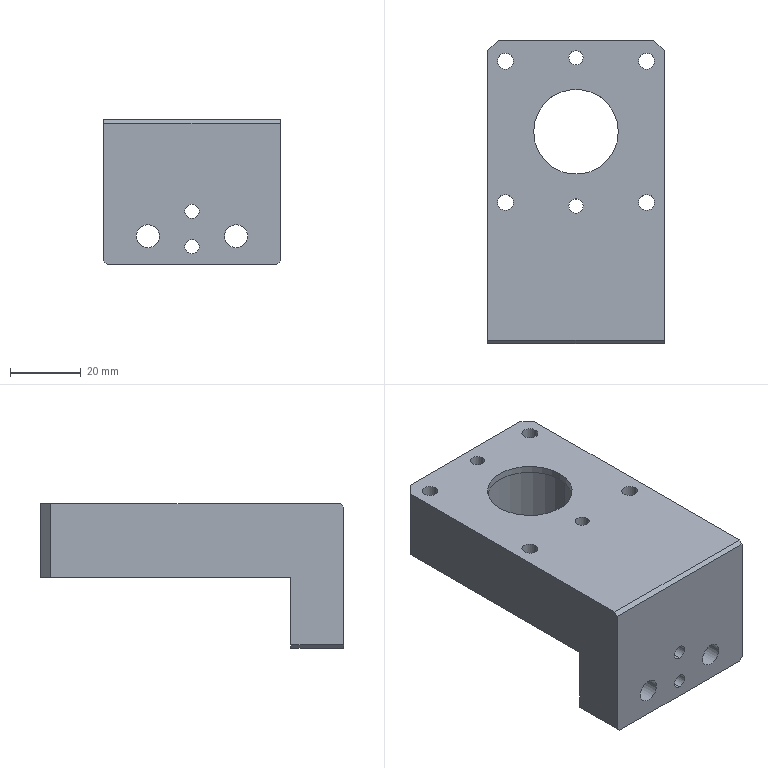Part | SolidWorks | features HoleWzd 4, ICE 3, Chamfer 2, Extrusion 1 | 1 solid | 58 faces | box 50 x 86 x 41 mm | volume 88498 mm3 | cylinder 36 | plane 18 | cone 4 | commonest cylinder face diameters 4 x8 4.5 x8 8 x8 2.5 x4 6.5 x4 24 x2